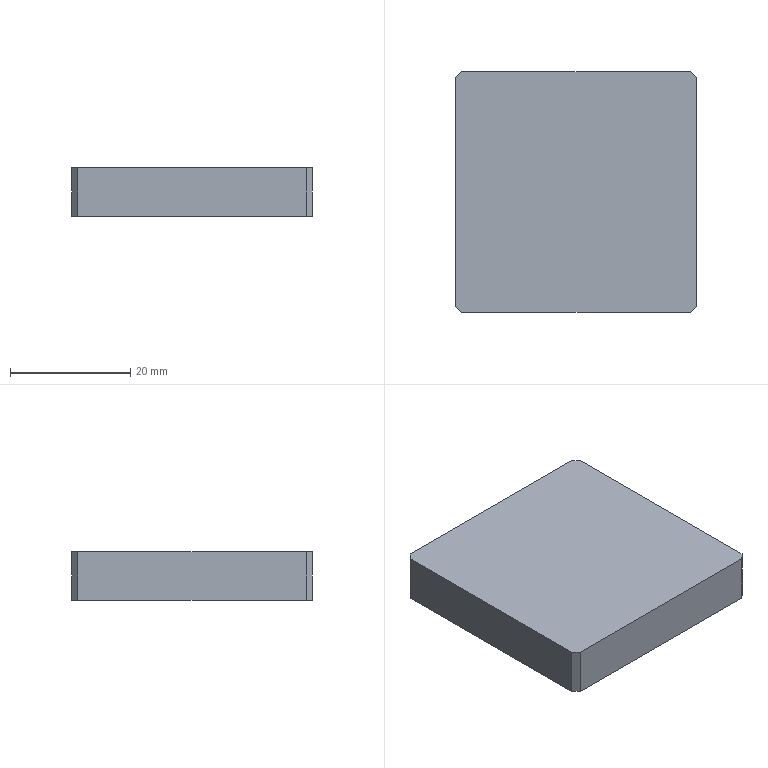Part | SolidWorks | features Chamfer 1, Extrusion 1 | 1 solid | 10 faces | box 40 x 40 x 8 mm | volume 12784 mm3 | plane 10
STEP:
#1=CARTESIAN_POINT('',(20.,-19.,8.));
#2=VERTEX_POINT('',#1);
#3=CARTESIAN_POINT('',(20.,19.,8.));
#4=VERTEX_POINT('',#3);
#5=CARTESIAN_POINT('',(20.,20.,8.));
#6=DIRECTION('',(0.,1.,0.));
#7=VECTOR('',#6,1000.);
#8=LINE('',#5,#7);
#9=EDGE_CURVE('',#2,#4,#8,.T.);
#10=ORIENTED_EDGE('',*,*,#9,.F.);
#11=CARTESIAN_POINT('',(20.,-19.,0.));
#12=VERTEX_POINT('',#11);
#13=CARTESIAN_POINT('',(20.,-19.,8.));
#14=DIRECTION('',(0.,0.,-1.));
#15=VECTOR('',#14,1000.);
#16=LINE('',#13,#15);
#17=EDGE_CURVE('',#2,#12,#16,.T.);
#18=ORIENTED_EDGE('',*,*,#17,.T.);
#19=CARTESIAN_POINT('',(20.,19.,0.));
#20=VERTEX_POINT('',#19);
#21=CARTESIAN_POINT('',(20.,20.,0.));
#22=DIRECTION('',(0.,1.,0.));
#23=VECTOR('',#22,1000.);
#24=LINE('',#21,#23);
#25=EDGE_CURVE('',#12,#20,#24,.T.);
#26=ORIENTED_EDGE('',*,*,#25,.T.);
#27=CARTESIAN_POINT('',(20.,19.,8.));
#28=DIRECTION('',(0.,0.,1.));
#29=VECTOR('',#28,1000.);
#30=LINE('',#27,#29);
#31=EDGE_CURVE('',#20,#4,#30,.T.);
#32=ORIENTED_EDGE('',*,*,#31,.T.);
#33=EDGE_LOOP('',(#10,#18,#26,#32));
#34=FACE_OUTER_BOUND('',#33,.T.);
#35=CARTESIAN_POINT('',(20.,20.,8.));
#36=DIRECTION('',(-1.,0.,0.));
#37=DIRECTION('',(0.,-1.,0.));
#38=AXIS2_PLACEMENT_3D('',#35,#36,#37);
#39=PLANE('',#38);
#40=ADVANCED_FACE('',(#34),#39,.F.);
#41=CARTESIAN_POINT('',(19.,20.,8.));
#42=VERTEX_POINT('',#41);
#43=CARTESIAN_POINT('',(-19.,20.,8.));
#44=VERTEX_POINT('',#43);
#45=CARTESIAN_POINT('',(-20.,20.,8.));
#46=DIRECTION('',(-1.,0.,0.));
#47=VECTOR('',#46,1000.);
#48=LINE('',#45,#47);
#49=EDGE_CURVE('',#42,#44,#48,.T.);
#50=ORIENTED_EDGE('',*,*,#49,.F.);
#51=CARTESIAN_POINT('',(19.,20.,0.));
#52=VERTEX_POINT('',#51);
#53=CARTESIAN_POINT('',(19.,20.,8.));
#54=DIRECTION('',(0.,0.,-1.));
#55=VECTOR('',#54,1000.);
#56=LINE('',#53,#55);
#57=EDGE_CURVE('',#42,#52,#56,.T.);
#58=ORIENTED_EDGE('',*,*,#57,.T.);
#59=CARTESIAN_POINT('',(-19.,20.,0.));
#60=VERTEX_POINT('',#59);
#61=CARTESIAN_POINT('',(-20.,20.,0.));
#62=DIRECTION('',(-1.,0.,0.));
#63=VECTOR('',#62,1000.);
#64=LINE('',#61,#63);
#65=EDGE_CURVE('',#52,#60,#64,.T.);
#66=ORIENTED_EDGE('',*,*,#65,.T.);
#67=CARTESIAN_POINT('',(-19.,20.,8.));
#68=DIRECTION('',(0.,0.,1.));
#69=VECTOR('',#68,1000.);
#70=LINE('',#67,#69);
#71=EDGE_CURVE('',#60,#44,#70,.T.);
#72=ORIENTED_EDGE('',*,*,#71,.T.);
#73=EDGE_LOOP('',(#50,#58,#66,#72));
#74=FACE_OUTER_BOUND('',#73,.T.);
#75=CARTESIAN_POINT('',(-20.,20.,8.));
#76=DIRECTION('',(0.,-1.,0.));
#77=DIRECTION('',(0.,0.,-1.));
#78=AXIS2_PLACEMENT_3D('',#75,#76,#77);
#79=PLANE('',#78);
#80=ADVANCED_FACE('',(#74),#79,.F.);
#81=CARTESIAN_POINT('',(-20.,19.,0.));
#82=VERTEX_POINT('',#81);
#83=CARTESIAN_POINT('',(-20.,-19.,0.));
#84=VERTEX_POINT('',#83);
#85=CARTESIAN_POINT('',(-20.,20.,0.));
#86=DIRECTION('',(0.,-1.,0.));
#87=VECTOR('',#86,1000.);
#88=LINE('',#85,#87);
#89=EDGE_CURVE('',#82,#84,#88,.T.);
#90=ORIENTED_EDGE('',*,*,#89,.T.);
#91=CARTESIAN_POINT('',(-20.,-19.,8.));
#92=VERTEX_POINT('',#91);
#93=CARTESIAN_POINT('',(-20.,-19.,8.));
#94=DIRECTION('',(0.,0.,1.));
#95=VECTOR('',#94,1000.);
#96=LINE('',#93,#95);
#97=EDGE_CURVE('',#84,#92,#96,.T.);
#98=ORIENTED_EDGE('',*,*,#97,.T.);
#99=CARTESIAN_POINT('',(-20.,19.,8.));
#100=VERTEX_POINT('',#99);
#101=CARTESIAN_POINT('',(-20.,20.,8.));
#102=DIRECTION('',(0.,-1.,0.));
#103=VECTOR('',#102,1000.);
#104=LINE('',#101,#103);
#105=EDGE_CURVE('',#100,#92,#104,.T.);
#106=ORIENTED_EDGE('',*,*,#105,.F.);
#107=CARTESIAN_POINT('',(-20.,19.,8.));
#108=DIRECTION('',(0.,0.,-1.));
#109=VECTOR('',#108,1000.);
#110=LINE('',#107,#109);
#111=EDGE_CURVE('',#100,#82,#110,.T.);
#112=ORIENTED_EDGE('',*,*,#111,.T.);
#113=EDGE_LOOP('',(#90,#98,#106,#112));
#114=FACE_OUTER_BOUND('',#113,.T.);
#115=CARTESIAN_POINT('',(-20.,20.,8.));
#116=DIRECTION('',(1.,0.,0.));
#117=DIRECTION('',(0.,1.,0.));
#118=AXIS2_PLACEMENT_3D('',#115,#116,#117);
#119=PLANE('',#118);
#120=ADVANCED_FACE('',(#114),#119,.F.);
#121=CARTESIAN_POINT('',(-19.,-20.,8.));
#122=VERTEX_POINT('',#121);
#123=CARTESIAN_POINT('',(19.,-20.,8.));
#124=VERTEX_POINT('',#123);
#125=CARTESIAN_POINT('',(-20.,-20.,8.));
#126=DIRECTION('',(1.,0.,0.));
#127=VECTOR('',#126,1000.);
#128=LINE('',#125,#127);
#129=EDGE_CURVE('',#122,#124,#128,.T.);
#130=ORIENTED_EDGE('',*,*,#129,.F.);
#131=CARTESIAN_POINT('',(-19.,-20.,0.));
#132=VERTEX_POINT('',#131);
#133=CARTESIAN_POINT('',(-19.,-20.,8.));
#134=DIRECTION('',(0.,0.,-1.));
#135=VECTOR('',#134,1000.);
#136=LINE('',#133,#135);
#137=EDGE_CURVE('',#122,#132,#136,.T.);
#138=ORIENTED_EDGE('',*,*,#137,.T.);
#139=CARTESIAN_POINT('',(19.,-20.,0.));
#140=VERTEX_POINT('',#139);
#141=CARTESIAN_POINT('',(-20.,-20.,0.));
#142=DIRECTION('',(1.,0.,0.));
#143=VECTOR('',#142,1000.);
#144=LINE('',#141,#143);
#145=EDGE_CURVE('',#132,#140,#144,.T.);
#146=ORIENTED_EDGE('',*,*,#145,.T.);
#147=CARTESIAN_POINT('',(19.,-20.,8.));
#148=DIRECTION('',(0.,0.,1.));
#149=VECTOR('',#148,1000.);
#150=LINE('',#147,#149);
#151=EDGE_CURVE('',#140,#124,#150,.T.);
#152=ORIENTED_EDGE('',*,*,#151,.T.);
#153=EDGE_LOOP('',(#130,#138,#146,#152));
#154=FACE_OUTER_BOUND('',#153,.T.);
#155=CARTESIAN_POINT('',(-20.,-20.,8.));
#156=DIRECTION('',(0.,1.,0.));
#157=DIRECTION('',(0.,0.,1.));
#158=AXIS2_PLACEMENT_3D('',#155,#156,#157);
#159=PLANE('',#158);
#160=ADVANCED_FACE('',(#154),#159,.F.);
#161=ORIENTED_EDGE('',*,*,#105,.T.);
#162=CARTESIAN_POINT('',(-19.5,-19.5,8.));
#163=DIRECTION('',(0.7071,-0.7071,0.));
#164=VECTOR('',#163,1000.);
#165=LINE('',#162,#164);
#166=EDGE_CURVE('',#92,#122,#165,.T.);
#167=ORIENTED_EDGE('',*,*,#166,.T.);
#168=ORIENTED_EDGE('',*,*,#129,.T.);
#169=CARTESIAN_POINT('',(19.5,-19.5,8.));
#170=DIRECTION('',(0.7071,0.7071,0.));
#171=VECTOR('',#170,1000.);
#172=LINE('',#169,#171);
#173=EDGE_CURVE('',#124,#2,#172,.T.);
#174=ORIENTED_EDGE('',*,*,#173,.T.);
#175=ORIENTED_EDGE('',*,*,#9,.T.);
#176=CARTESIAN_POINT('',(19.5,19.5,8.));
#177=DIRECTION('',(-0.7071,0.7071,0.));
#178=VECTOR('',#177,1000.);
#179=LINE('',#176,#178);
#180=EDGE_CURVE('',#4,#42,#179,.T.);
#181=ORIENTED_EDGE('',*,*,#180,.T.);
#182=ORIENTED_EDGE('',*,*,#49,.T.);
#183=CARTESIAN_POINT('',(-19.5,19.5,8.));
#184=DIRECTION('',(-0.7071,-0.7071,0.));
#185=VECTOR('',#184,1000.);
#186=LINE('',#183,#185);
#187=EDGE_CURVE('',#44,#100,#186,.T.);
#188=ORIENTED_EDGE('',*,*,#187,.T.);
#189=EDGE_LOOP('',(#161,#167,#168,#174,#175,#181,#182,#188));
#190=FACE_OUTER_BOUND('',#189,.T.);
#191=CARTESIAN_POINT('',(0.,0.,8.));
#192=DIRECTION('',(0.,0.,1.));
#193=DIRECTION('',(1.,0.,0.));
#194=AXIS2_PLACEMENT_3D('',#191,#192,#193);
#195=PLANE('',#194);
#196=ADVANCED_FACE('',(#190),#195,.T.);
#197=ORIENTED_EDGE('',*,*,#145,.F.);
#198=CARTESIAN_POINT('',(-19.,-20.,0.));
#199=DIRECTION('',(-0.7071,0.7071,0.));
#200=VECTOR('',#199,1000.);
#201=LINE('',#198,#200);
#202=EDGE_CURVE('',#132,#84,#201,.T.);
#203=ORIENTED_EDGE('',*,*,#202,.T.);
#204=ORIENTED_EDGE('',*,*,#89,.F.);
#205=CARTESIAN_POINT('',(-20.,19.,0.));
#206=DIRECTION('',(0.7071,0.7071,0.));
#207=VECTOR('',#206,1000.);
#208=LINE('',#205,#207);
#209=EDGE_CURVE('',#82,#60,#208,.T.);
#210=ORIENTED_EDGE('',*,*,#209,.T.);
#211=ORIENTED_EDGE('',*,*,#65,.F.);
#212=CARTESIAN_POINT('',(19.,20.,0.));
#213=DIRECTION('',(0.7071,-0.7071,0.));
#214=VECTOR('',#213,1000.);
#215=LINE('',#212,#214);
#216=EDGE_CURVE('',#52,#20,#215,.T.);
#217=ORIENTED_EDGE('',*,*,#216,.T.);
#218=ORIENTED_EDGE('',*,*,#25,.F.);
#219=CARTESIAN_POINT('',(20.,-19.,0.));
#220=DIRECTION('',(-0.7071,-0.7071,0.));
#221=VECTOR('',#220,1000.);
#222=LINE('',#219,#221);
#223=EDGE_CURVE('',#12,#140,#222,.T.);
#224=ORIENTED_EDGE('',*,*,#223,.T.);
#225=EDGE_LOOP('',(#197,#203,#204,#210,#211,#217,#218,#224));
#226=FACE_OUTER_BOUND('',#225,.T.);
#227=CARTESIAN_POINT('',(0.,0.,0.));
#228=DIRECTION('',(0.,0.,1.));
#229=DIRECTION('',(1.,0.,0.));
#230=AXIS2_PLACEMENT_3D('',#227,#228,#229);
#231=PLANE('',#230);
#232=ADVANCED_FACE('',(#226),#231,.F.);
#233=ORIENTED_EDGE('',*,*,#166,.F.);
#234=ORIENTED_EDGE('',*,*,#97,.F.);
#235=ORIENTED_EDGE('',*,*,#202,.F.);
#236=ORIENTED_EDGE('',*,*,#137,.F.);
#237=EDGE_LOOP('',(#233,#234,#235,#236));
#238=FACE_OUTER_BOUND('',#237,.T.);
#239=CARTESIAN_POINT('',(-19.,-20.,8.));
#240=DIRECTION('',(0.7071,0.7071,0.));
#241=DIRECTION('',(0.,0.,-1.));
#242=AXIS2_PLACEMENT_3D('',#239,#240,#241);
#243=PLANE('',#242);
#244=ADVANCED_FACE('',(#238),#243,.F.);
#245=ORIENTED_EDGE('',*,*,#173,.F.);
#246=ORIENTED_EDGE('',*,*,#151,.F.);
#247=ORIENTED_EDGE('',*,*,#223,.F.);
#248=ORIENTED_EDGE('',*,*,#17,.F.);
#249=EDGE_LOOP('',(#245,#246,#247,#248));
#250=FACE_OUTER_BOUND('',#249,.T.);
#251=CARTESIAN_POINT('',(20.,-19.,8.));
#252=DIRECTION('',(-0.7071,0.7071,0.));
#253=DIRECTION('',(0.,0.,-1.));
#254=AXIS2_PLACEMENT_3D('',#251,#252,#253);
#255=PLANE('',#254);
#256=ADVANCED_FACE('',(#250),#255,.F.);
#257=ORIENTED_EDGE('',*,*,#180,.F.);
#258=ORIENTED_EDGE('',*,*,#31,.F.);
#259=ORIENTED_EDGE('',*,*,#216,.F.);
#260=ORIENTED_EDGE('',*,*,#57,.F.);
#261=EDGE_LOOP('',(#257,#258,#259,#260));
#262=FACE_OUTER_BOUND('',#261,.T.);
#263=CARTESIAN_POINT('',(19.,20.,8.));
#264=DIRECTION('',(-0.7071,-0.7071,0.));
#265=DIRECTION('',(0.,0.,-1.));
#266=AXIS2_PLACEMENT_3D('',#263,#264,#265);
#267=PLANE('',#266);
#268=ADVANCED_FACE('',(#262),#267,.F.);
#269=ORIENTED_EDGE('',*,*,#187,.F.);
#270=ORIENTED_EDGE('',*,*,#71,.F.);
#271=ORIENTED_EDGE('',*,*,#209,.F.);
#272=ORIENTED_EDGE('',*,*,#111,.F.);
#273=EDGE_LOOP('',(#269,#270,#271,#272));
#274=FACE_OUTER_BOUND('',#273,.T.);
#275=CARTESIAN_POINT('',(-20.,19.,8.));
#276=DIRECTION('',(0.7071,-0.7071,0.));
#277=DIRECTION('',(0.,0.,-1.));
#278=AXIS2_PLACEMENT_3D('',#275,#276,#277);
#279=PLANE('',#278);
#280=ADVANCED_FACE('',(#274),#279,.F.);
#281=CLOSED_SHELL('',(#40,#80,#120,#160,#196,#232,#244,#256,#268,#280));
#282=MANIFOLD_SOLID_BREP('',#281);
#283=CARTESIAN_POINT('',(0.,0.,0.));
#284=DIRECTION('',(0.,0.,1.));
#285=DIRECTION('',(1.,0.,0.));
#286=AXIS2_PLACEMENT_3D('',#283,#284,#285);
#287=(LENGTH_UNIT()NAMED_UNIT(*)SI_UNIT(.MILLI.,.METRE.));
#288=UNCERTAINTY_MEASURE_WITH_UNIT(LENGTH_MEASURE(0.00001),#287,'','');
#289=(NAMED_UNIT(*)PLANE_ANGLE_UNIT()SI_UNIT($,.RADIAN.));
#290=(NAMED_UNIT(*)SI_UNIT($,.STERADIAN.)SOLID_ANGLE_UNIT());
#291=(GEOMETRIC_REPRESENTATION_CONTEXT(3)GLOBAL_UNCERTAINTY_ASSIGNED_CONTEXT((#288))GLOBAL_UNIT_ASSIGNED_CONTEXT((#287,#289,#290))REPRESENTATION_CONTEXT('',''));
#292=ADVANCED_BREP_SHAPE_REPRESENTATION('',(#282,#286),#291);